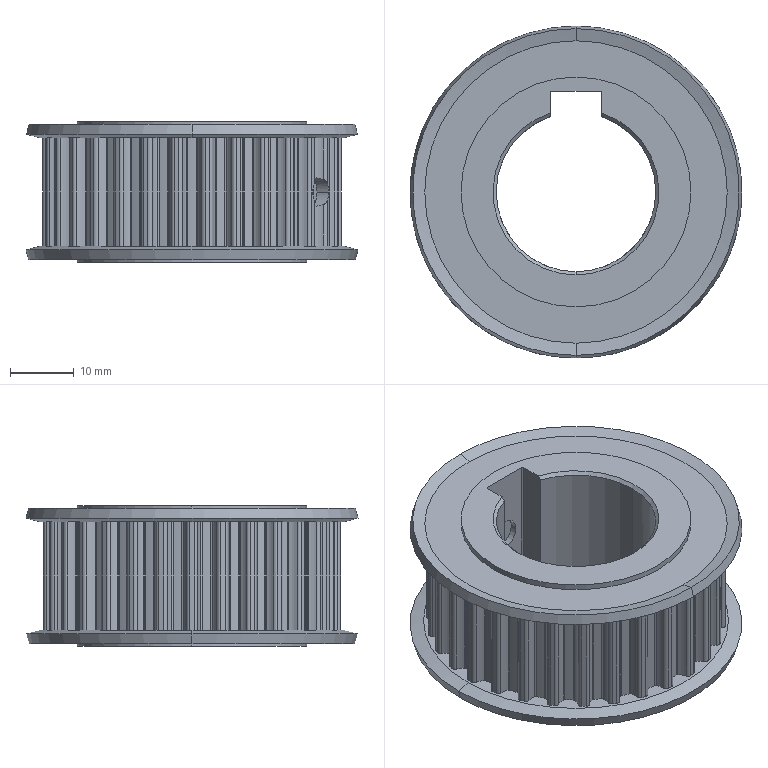Part | SolidWorks | features BaseBody 1 | 1 solid | 341 faces | box 52 x 52 x 22 mm | volume 23799 mm3 | cylinder 297 | plane 27 | cone 17 | commonest cylinder face diameters 1.1 x77 0.5 x72 6.55 x68 43.25 x32 46.79 x31 4.917 x8